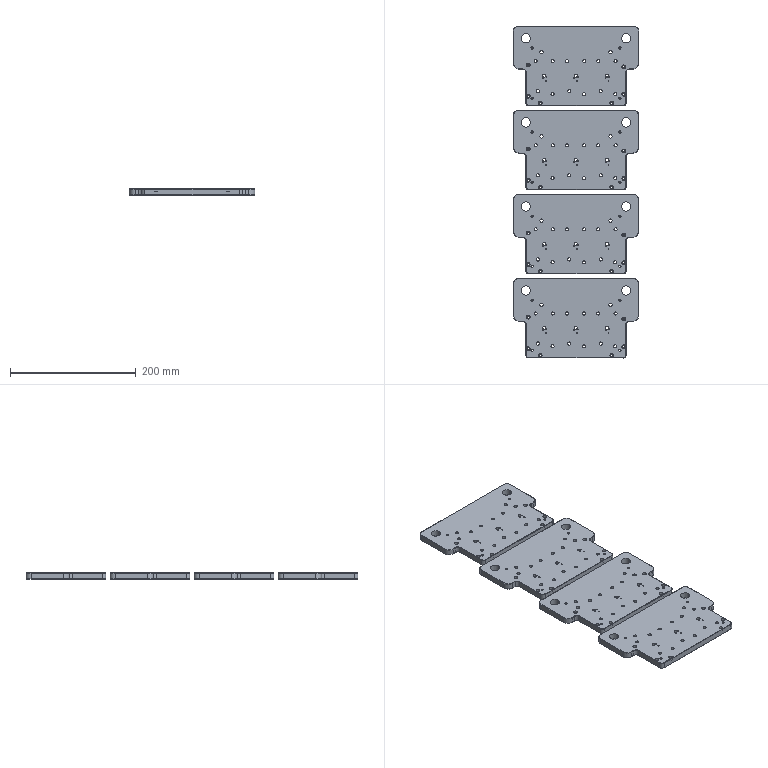NC program | NX | posted with a generic post | part box 200 x 529 x 10 mm
Lines 1504 to 1801 of 1801:
(刀补 , TOOL : D3)
N2940 T03 M6
N2942 G54
N2944 G17 G0 G90 X-55. Y21.5 S9500 M3
N2946 G43 Z30. H3
N2948 Z-1.5
N2950 G41 G94 G1 X-55.004 Y21.6 F1000. D3
N2952 G3 X-55.95 Y21.5 R0.478
N2954 X-55.95 Y21.5 Z-3. I0.95 J0.
N2956 X-55.95 Y21.5 Z-4.5 I0.95 J0.
N2958 X-55.95 Y21.5 Z-6. I0.95 J0.
N2960 X-55.95 Y21.5 Z-7.5 I0.95 J0.
N2962 X-55.95 Y21.5 Z-9. I0.95 J0.
N2964 X-54.525 Y22.323 Z-10. R-0.95
N2966 X-55.823 Y21.975 R0.95
N2968 X-54.525 Y22.323 R-0.95
N2970 X-55.085 Y21.553 R0.478
N2972 G40
N2974 G1 X-55. Y21.5
N2976 G0 Z30.
N2978 X55.
N2980 Z-1.5
N2982 G41 G1 X54.996 Y21.6
N2984 G3 X54.05 Y21.5 R0.478
N2986 X54.05 Y21.5 Z-3. I0.95 J0.
N2988 X54.05 Y21.5 Z-4.5 I0.95 J0.
N2990 X54.05 Y21.5 Z-6. I0.95 J0.
N2992 X54.05 Y21.5 Z-7.5 I0.95 J0.
N2994 X54.05 Y21.5 Z-9. I0.95 J0.
N2996 X55.475 Y22.323 Z-10. R-0.95
N2998 X54.177 Y21.975 R0.95
N3000 X55.475 Y22.323 R-0.95
N3002 X54.915 Y21.553 R0.478
N3004 G40
N3006 G1 X55. Y21.5
N3008 G0 Z30.
(刀补_COPY , TOOL : D3)
N3010 X-63.044 Y7.4
N3012 Z0.5
N3014 G41 G1 X-63.048 Y7.5
N3016 G3 X-63.994 Y7.4 R0.478
N3018 X-63.994 Y7.4 Z-1. I0.95 J0.
N3020 X-63.994 Y7.4 Z-2.5 I0.95 J0.
N3022 X-63.994 Y7.4 Z-4. I0.95 J0.
N3024 X-63.994 Y7.4 Z-5.5 I0.95 J0.
N3026 X-63.994 Y7.4 Z-7. I0.95 J0.
N3028 X-63.994 Y7.4 Z-8.5 I0.95 J0.
N3030 X-63.994 Y7.4 Z-10. I0.95 J0.
N3032 X-63.044 Y6.45 R0.95
N3034 X-63.994 Y7.4 R-0.95
N3036 X-63.048 Y7.3 R0.478
N3038 G40
N3040 G1 X-63.044 Y7.4
N3042 G0 Z30.
N3044 X-35.603 Y7.41
N3046 Z0.5
N3048 G41 G1 X-35.607 Y7.51
N3050 G3 X-36.553 Y7.41 R0.478
N3052 X-36.553 Y7.41 Z-1. I0.95 J0.
N3054 X-36.553 Y7.41 Z-2.5 I0.95 J0.
N3056 X-36.553 Y7.41 Z-4. I0.95 J0.
N3058 X-36.553 Y7.41 Z-5.5 I0.95 J0.
N3060 X-36.553 Y7.41 Z-7. I0.95 J0.
N3062 X-36.553 Y7.41 Z-8.5 I0.95 J0.
N3064 X-36.553 Y7.41 Z-10. I0.95 J0.
N3066 X-35.603 Y6.46 R0.95
N3068 X-36.553 Y7.41 R-0.95
N3070 X-35.607 Y7.311 R0.478
N3072 G40
N3074 G1 X-35.603 Y7.41
N3076 G0 Z30.
N3078 X-13.044 Y7.4
N3080 Z0.5
N3082 G41 G1 X-13.048 Y7.5
N3084 G3 X-13.994 Y7.4 R0.478
N3086 X-13.994 Y7.4 Z-1. I0.95 J0.
N3088 X-13.994 Y7.4 Z-2.5 I0.95 J0.
N3090 X-13.994 Y7.4 Z-4. I0.95 J0.
N3092 X-13.994 Y7.4 Z-5.5 I0.95 J0.
N3094 X-13.994 Y7.4 Z-7. I0.95 J0.
N3096 X-13.994 Y7.4 Z-8.5 I0.95 J0.
N3098 X-13.994 Y7.4 Z-10. I0.95 J0.
N3100 X-13.044 Y6.45 R0.95
N3102 X-13.994 Y7.4 R-0.95
N3104 X-13.048 Y7.3 R0.478
N3106 G40
N3108 G1 X-13.044 Y7.4
N3110 G0 Z30.
N3112 X14.397 Y7.41
N3114 Z0.5
N3116 G41 G1 X14.393 Y7.51
N3118 G3 X13.447 Y7.41 R0.478
N3120 X13.447 Y7.41 Z-1. I0.95 J0.
N3122 X13.447 Y7.41 Z-2.5 I0.95 J0.
N3124 X13.447 Y7.41 Z-4. I0.95 J0.
N3126 X13.447 Y7.41 Z-5.5 I0.95 J0.
N3128 X13.447 Y7.41 Z-7. I0.95 J0.
N3130 X13.447 Y7.41 Z-8.5 I0.95 J0.
N3132 X13.447 Y7.41 Z-10. I0.95 J0.
N3134 X14.397 Y6.46 R0.95
N3136 X13.447 Y7.41 R-0.95
N3138 X14.393 Y7.311 R0.478
N3140 G40
N3142 G1 X14.397 Y7.41
N3144 G0 Z30.
N3146 X36.956 Y7.4
N3148 Z0.5
N3150 G41 G1 X36.952 Y7.5
N3152 G3 X36.006 Y7.4 R0.478
N3154 X36.006 Y7.4 Z-1. I0.95 J0.
N3156 X36.006 Y7.4 Z-2.5 I0.95 J0.
N3158 X36.006 Y7.4 Z-4. I0.95 J0.
N3160 X36.006 Y7.4 Z-5.5 I0.95 J0.
N3162 X36.006 Y7.4 Z-7. I0.95 J0.
N3164 X36.006 Y7.4 Z-8.5 I0.95 J0.
N3166 X36.006 Y7.4 Z-10. I0.95 J0.
N3168 X36.956 Y6.45 R0.95
N3170 X36.006 Y7.4 R-0.95
N3172 X36.952 Y7.3 R0.478
N3174 G40
N3176 G1 X36.956 Y7.4
N3178 G0 Z30.
N3180 X64.397 Y7.41
N3182 Z0.5
N3184 G41 G1 X64.393 Y7.51
N3186 G3 X63.447 Y7.41 R0.478
N3188 X63.447 Y7.41 Z-1. I0.95 J0.
N3190 X63.447 Y7.41 Z-2.5 I0.95 J0.
N3192 X63.447 Y7.41 Z-4. I0.95 J0.
N3194 X63.447 Y7.41 Z-5.5 I0.95 J0.
N3196 X63.447 Y7.41 Z-7. I0.95 J0.
N3198 X63.447 Y7.41 Z-8.5 I0.95 J0.
N3200 X63.447 Y7.41 Z-10. I0.95 J0.
N3202 X64.397 Y6.46 R0.95
N3204 X63.447 Y7.41 R-0.95
N3206 X64.393 Y7.311 R0.478
N3208 G40
N3210 G1 X64.397 Y7.41
N3212 G0 Z30.
N3214 X50.608 Y-15.627
N3216 Z0.5
N3218 G41 G1 X50.604 Y-15.527
N3220 G3 X49.658 Y-15.627 R0.478
N3222 X49.658 Y-15.627 Z-1. I0.95 J0.
N3224 X49.658 Y-15.627 Z-2.5 I0.95 J0.
N3226 X49.658 Y-15.627 Z-4. I0.95 J0.
N3228 X49.658 Y-15.627 Z-5.5 I0.95 J0.
N3230 X49.658 Y-15.627 Z-7. I0.95 J0.
N3232 X49.658 Y-15.627 Z-8.5 I0.95 J0.
N3234 X49.658 Y-15.627 Z-10. I0.95 J0.
N3236 X50.608 Y-16.577 R0.95
N3238 X49.658 Y-15.627 R-0.95
N3240 X50.604 Y-15.727 R0.478
N3242 G40
N3244 G1 X50.608 Y-15.627
N3246 G0 Z30.
N3248 X0.608
N3250 Z0.5
N3252 G41 G1 X0.604 Y-15.527
N3254 G3 X-0.342 Y-15.627 R0.478
N3256 X-0.342 Y-15.627 Z-1. I0.95 J0.
N3258 X-0.342 Y-15.627 Z-2.5 I0.95 J0.
N3260 X-0.342 Y-15.627 Z-4. I0.95 J0.
N3262 X-0.342 Y-15.627 Z-5.5 I0.95 J0.
N3264 X-0.342 Y-15.627 Z-7. I0.95 J0.
N3266 X-0.342 Y-15.627 Z-8.5 I0.95 J0.
N3268 X-0.342 Y-15.627 Z-10. I0.95 J0.
N3270 X0.608 Y-16.577 R0.95
N3272 X-0.342 Y-15.627 R-0.95
N3274 X0.604 Y-15.727 R0.478
N3276 G40
N3278 G1 X0.608 Y-15.627
N3280 G0 Z30.
N3282 X-49.392
N3284 Z0.5
N3286 G41 G1 X-49.396 Y-15.527
N3288 G3 X-50.342 Y-15.627 R0.478
N3290 X-50.342 Y-15.627 Z-1. I0.95 J0.
N3292 X-50.342 Y-15.627 Z-2.5 I0.95 J0.
N3294 X-50.342 Y-15.627 Z-4. I0.95 J0.
N3296 X-50.342 Y-15.627 Z-5.5 I0.95 J0.
N3298 X-50.342 Y-15.627 Z-7. I0.95 J0.
N3300 X-50.342 Y-15.627 Z-8.5 I0.95 J0.
N3302 X-50.342 Y-15.627 Z-10. I0.95 J0.
N3304 X-49.392 Y-16.577 R0.95
N3306 X-50.342 Y-15.627 R-0.95
N3308 X-49.396 Y-15.727 R0.478
N3310 G40
N3312 G1 X-49.392 Y-15.627
N3314 G0 Z30.
N3316 X-62.621 Y-45.039
N3318 Z0.5
N3320 G41 G1 X-62.625 Y-44.939
N3322 G3 X-63.571 Y-45.039 R0.478
N3324 X-63.571 Y-45.039 Z-1. I0.95 J0.
N3326 X-63.571 Y-45.039 Z-2.5 I0.95 J0.
N3328 X-63.571 Y-45.039 Z-4. I0.95 J0.
N3330 X-63.571 Y-45.039 Z-5.5 I0.95 J0.
N3332 X-63.571 Y-45.039 Z-7. I0.95 J0.
N3334 X-63.571 Y-45.039 Z-8.5 I0.95 J0.
N3336 X-63.571 Y-45.039 Z-10. I0.95 J0.
N3338 X-62.621 Y-45.989 R0.95
N3340 X-63.571 Y-45.039 R-0.95
N3342 X-62.625 Y-45.139 R0.478
N3344 G40
N3346 G1 X-62.621 Y-45.039
N3348 G0 Z30.
N3350 X-39.273 Y-40.475
N3352 Z0.5
N3354 G41 G1 X-39.277 Y-40.375
N3356 G3 X-40.223 Y-40.475 R0.478
N3358 X-40.223 Y-40.475 Z-1. I0.95 J0.
N3360 X-40.223 Y-40.475 Z-2.5 I0.95 J0.
N3362 X-40.223 Y-40.475 Z-4. I0.95 J0.
N3364 X-40.223 Y-40.475 Z-5.5 I0.95 J0.
N3366 X-40.223 Y-40.475 Z-7. I0.95 J0.
N3368 X-40.223 Y-40.475 Z-8.5 I0.95 J0.
N3370 X-40.223 Y-40.475 Z-10. I0.95 J0.
N3372 X-39.273 Y-41.425 R0.95
N3374 X-40.223 Y-40.475 R-0.95
N3376 X-39.277 Y-40.575 R0.478
N3378 G40
N3380 G1 X-39.273 Y-40.475
N3382 G0 Z30.
N3384 X-12.621 Y-45.039
N3386 Z0.5
N3388 G41 G1 X-12.625 Y-44.939
N3390 G3 X-13.571 Y-45.039 R0.478
N3392 X-13.571 Y-45.039 Z-1. I0.95 J0.
N3394 X-13.571 Y-45.039 Z-2.5 I0.95 J0.
N3396 X-13.571 Y-45.039 Z-4. I0.95 J0.
N3398 X-13.571 Y-45.039 Z-5.5 I0.95 J0.
N3400 X-13.571 Y-45.039 Z-7. I0.95 J0.
N3402 X-13.571 Y-45.039 Z-8.5 I0.95 J0.
N3404 X-13.571 Y-45.039 Z-10. I0.95 J0.
N3406 X-12.621 Y-45.989 R0.95
N3408 X-13.571 Y-45.039 R-0.95
N3410 X-12.625 Y-45.139 R0.478
N3412 G40
N3414 G1 X-12.621 Y-45.039
N3416 G0 Z30.
N3418 X10.727 Y-40.475
N3420 Z0.5
N3422 G41 G1 X10.723 Y-40.375
N3424 G3 X9.777 Y-40.475 R0.478
N3426 X9.777 Y-40.475 Z-1. I0.95 J0.
N3428 X9.777 Y-40.475 Z-2.5 I0.95 J0.
N3430 X9.777 Y-40.475 Z-4. I0.95 J0.
N3432 X9.777 Y-40.475 Z-5.5 I0.95 J0.
N3434 X9.777 Y-40.475 Z-7. I0.95 J0.
N3436 X9.777 Y-40.475 Z-8.5 I0.95 J0.
N3438 X9.777 Y-40.475 Z-10. I0.95 J0.
N3440 X10.727 Y-41.425 R0.95
N3442 X9.777 Y-40.475 R-0.95
N3444 X10.723 Y-40.575 R0.478
N3446 G40
N3448 G1 X10.727 Y-40.475
N3450 G0 Z30.
N3452 X37.379 Y-45.039
N3454 Z0.5
N3456 G41 G1 X37.375 Y-44.939
N3458 G3 X36.429 Y-45.039 R0.478
N3460 X36.429 Y-45.039 Z-1. I0.95 J0.
N3462 X36.429 Y-45.039 Z-2.5 I0.95 J0.
N3464 X36.429 Y-45.039 Z-4. I0.95 J0.
N3466 X36.429 Y-45.039 Z-5.5 I0.95 J0.
N3468 X36.429 Y-45.039 Z-7. I0.95 J0.
N3470 X36.429 Y-45.039 Z-8.5 I0.95 J0.
N3472 X36.429 Y-45.039 Z-10. I0.95 J0.
N3474 X37.379 Y-45.989 R0.95
N3476 X36.429 Y-45.039 R-0.95
N3478 X37.375 Y-45.139 R0.478
N3480 G40
N3482 G1 X37.379 Y-45.039
N3484 G0 Z30.
N3486 X60.727 Y-40.475
N3488 Z0.5
N3490 G41 G1 X60.723 Y-40.375
N3492 G3 X59.777 Y-40.475 R0.478
N3494 X59.777 Y-40.475 Z-1. I0.95 J0.
N3496 X59.777 Y-40.475 Z-2.5 I0.95 J0.
N3498 X59.777 Y-40.475 Z-4. I0.95 J0.
N3500 X59.777 Y-40.475 Z-5.5 I0.95 J0.
N3502 X59.777 Y-40.475 Z-7. I0.95 J0.
N3504 X59.777 Y-40.475 Z-8.5 I0.95 J0.
N3506 X59.777 Y-40.475 Z-10. I0.95 J0.
N3508 X60.727 Y-41.425 R0.95
N3510 X59.777 Y-40.475 R-0.95
N3512 X60.723 Y-40.575 R0.478
N3514 G40
N3516 G1 X60.727 Y-40.475
N3518 G0 Z30.
N3520 M5
N3522 M2